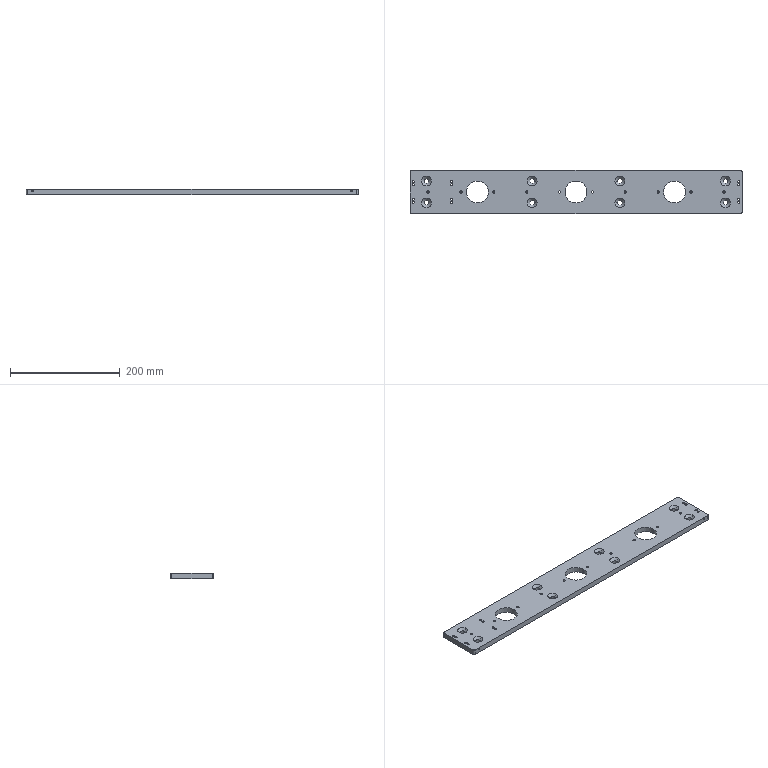Part | STEP file | PN_0050 | 1 solid | 100 faces | box 606 x 80 x 10 mm | volume 436139 mm3 | cylinder 74 | cone 20 | plane 6 | commonest cylinder face diameters 4.2 x20 9 x16 3.3 x12 4 x12 40 x6 2.5 x4